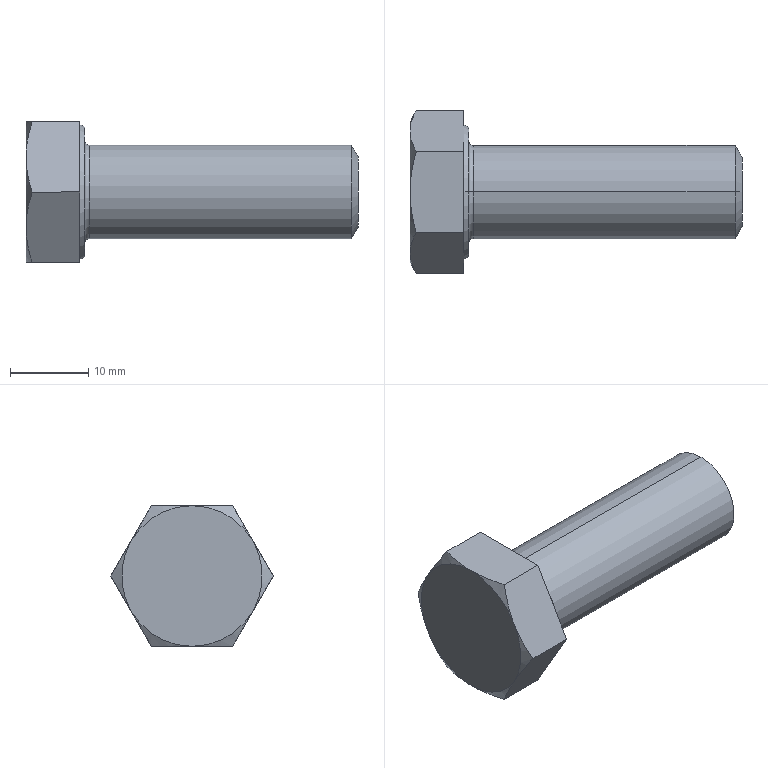Part | SolidWorks | features RevCut 3, Extrusion 1, Fillet 1, LPattern 1, Revolution 1 | 1 solid | 24 faces | box 42.5 x 20.785 x 18 mm | volume 6004 mm3 | cone 10 | plane 10 | torus 2 | cylinder 2 | commonest cylinder face diameters 12 x2
STEP:
#1=CARTESIAN_POINT('',(42.5,0.,4.484));
#2=VERTEX_POINT('',#1);
#3=CARTESIAN_POINT('',(42.5,0.,-4.484));
#4=VERTEX_POINT('',#3);
#5=CARTESIAN_POINT('',(42.5,0.,0.));
#6=DIRECTION('',(-1.,0.,0.));
#7=DIRECTION('',(0.,0.,1.));
#8=AXIS2_PLACEMENT_3D('',#5,#6,#7);
#9=CIRCLE('',#8,4.484);
#10=EDGE_CURVE('',#2,#4,#9,.T.);
#11=ORIENTED_EDGE('',*,*,#10,.T.);
#12=CARTESIAN_POINT('',(41.625,0.,-6.));
#13=VERTEX_POINT('',#12);
#14=CARTESIAN_POINT('',(41.625,0.,-6.));
#15=DIRECTION('',(-0.5,0.,-0.866));
#16=VECTOR('',#15,1000.);
#17=LINE('',#14,#16);
#18=EDGE_CURVE('',#4,#13,#17,.T.);
#19=ORIENTED_EDGE('',*,*,#18,.T.);
#20=CARTESIAN_POINT('',(41.625,0.,6.));
#21=VERTEX_POINT('',#20);
#22=CARTESIAN_POINT('',(41.625,0.,0.));
#23=DIRECTION('',(-1.,0.,0.));
#24=DIRECTION('',(0.,0.,1.));
#25=AXIS2_PLACEMENT_3D('',#22,#23,#24);
#26=CIRCLE('',#25,6.);
#27=EDGE_CURVE('',#21,#13,#26,.T.);
#28=ORIENTED_EDGE('',*,*,#27,.F.);
#29=CARTESIAN_POINT('',(41.625,0.,6.));
#30=DIRECTION('',(-0.5,0.,0.866));
#31=VECTOR('',#30,1000.);
#32=LINE('',#29,#31);
#33=EDGE_CURVE('',#2,#21,#32,.T.);
#34=ORIENTED_EDGE('',*,*,#33,.F.);
#35=EDGE_LOOP('',(#11,#19,#28,#34));
#36=FACE_OUTER_BOUND('',#35,.T.);
#37=CARTESIAN_POINT('',(41.625,0.,0.));
#38=DIRECTION('',(-1.,0.,0.));
#39=DIRECTION('',(0.,0.,1.));
#40=AXIS2_PLACEMENT_3D('',#37,#38,#39);
#41=CONICAL_SURFACE('',#40,6.,1.047);
#42=ADVANCED_FACE('',(#36),#41,.T.);
#43=CARTESIAN_POINT('',(8.1,0.,6.));
#44=VERTEX_POINT('',#43);
#45=CARTESIAN_POINT('',(8.1,0.,-6.));
#46=VERTEX_POINT('',#45);
#47=CARTESIAN_POINT('',(8.1,0.,0.));
#48=DIRECTION('',(1.,0.,0.));
#49=DIRECTION('',(0.,0.,-1.));
#50=AXIS2_PLACEMENT_3D('',#47,#48,#49);
#51=CIRCLE('',#50,6.);
#52=EDGE_CURVE('',#44,#46,#51,.T.);
#53=ORIENTED_EDGE('',*,*,#52,.F.);
#54=CARTESIAN_POINT('',(7.5,0.,6.6));
#55=VERTEX_POINT('',#54);
#56=CARTESIAN_POINT('',(8.1,0.,6.6));
#57=DIRECTION('',(0.,1.,0.));
#58=DIRECTION('',(0.,0.,1.));
#59=AXIS2_PLACEMENT_3D('',#56,#57,#58);
#60=CIRCLE('',#59,0.6);
#61=EDGE_CURVE('',#44,#55,#60,.T.);
#62=ORIENTED_EDGE('',*,*,#61,.T.);
#63=CARTESIAN_POINT('',(7.5,0.,-6.6));
#64=VERTEX_POINT('',#63);
#65=CARTESIAN_POINT('',(7.5,0.,0.));
#66=DIRECTION('',(-1.,0.,0.));
#67=DIRECTION('',(0.,0.,-1.));
#68=AXIS2_PLACEMENT_3D('',#65,#66,#67);
#69=CIRCLE('',#68,6.6);
#70=EDGE_CURVE('',#64,#55,#69,.T.);
#71=ORIENTED_EDGE('',*,*,#70,.F.);
#72=CARTESIAN_POINT('',(8.1,0.,-6.6));
#73=DIRECTION('',(0.,-1.,0.));
#74=DIRECTION('',(0.,0.,-1.));
#75=AXIS2_PLACEMENT_3D('',#72,#73,#74);
#76=CIRCLE('',#75,0.6);
#77=EDGE_CURVE('',#46,#64,#76,.T.);
#78=ORIENTED_EDGE('',*,*,#77,.F.);
#79=EDGE_LOOP('',(#53,#62,#71,#78));
#80=FACE_OUTER_BOUND('',#79,.T.);
#81=CARTESIAN_POINT('',(8.1,0.,0.));
#82=DIRECTION('',(1.,0.,0.));
#83=DIRECTION('',(0.,0.,-1.));
#84=AXIS2_PLACEMENT_3D('',#81,#82,#83);
#85=TOROIDAL_SURFACE('',#84,6.6,0.6);
#86=ADVANCED_FACE('',(#80),#85,.F.);
#87=CARTESIAN_POINT('',(7.5,0.,8.315));
#88=VERTEX_POINT('',#87);
#89=CARTESIAN_POINT('',(7.5,0.,-8.315));
#90=VERTEX_POINT('',#89);
#91=CARTESIAN_POINT('',(7.5,0.,0.));
#92=DIRECTION('',(-1.,0.,0.));
#93=DIRECTION('',(0.,0.,1.));
#94=AXIS2_PLACEMENT_3D('',#91,#92,#93);
#95=CIRCLE('',#94,8.315);
#96=EDGE_CURVE('',#88,#90,#95,.T.);
#97=ORIENTED_EDGE('',*,*,#96,.T.);
#98=CARTESIAN_POINT('',(6.9,0.,-8.661));
#99=VERTEX_POINT('',#98);
#100=CARTESIAN_POINT('',(6.9,0.,-8.661));
#101=DIRECTION('',(-0.866,0.,-0.5));
#102=VECTOR('',#101,1000.);
#103=LINE('',#100,#102);
#104=EDGE_CURVE('',#90,#99,#103,.T.);
#105=ORIENTED_EDGE('',*,*,#104,.T.);
#106=CARTESIAN_POINT('',(6.9,0.,8.661));
#107=VERTEX_POINT('',#106);
#108=CARTESIAN_POINT('',(6.9,0.,0.));
#109=DIRECTION('',(-1.,0.,0.));
#110=DIRECTION('',(0.,0.,1.));
#111=AXIS2_PLACEMENT_3D('',#108,#109,#110);
#112=CIRCLE('',#111,8.661);
#113=EDGE_CURVE('',#107,#99,#112,.T.);
#114=ORIENTED_EDGE('',*,*,#113,.F.);
#115=CARTESIAN_POINT('',(6.9,0.,8.661));
#116=DIRECTION('',(-0.866,0.,0.5));
#117=VECTOR('',#116,1000.);
#118=LINE('',#115,#117);
#119=EDGE_CURVE('',#88,#107,#118,.T.);
#120=ORIENTED_EDGE('',*,*,#119,.F.);
#121=EDGE_LOOP('',(#97,#105,#114,#120));
#122=FACE_OUTER_BOUND('',#121,.T.);
#123=CARTESIAN_POINT('',(6.9,0.,0.));
#124=DIRECTION('',(-1.,0.,0.));
#125=DIRECTION('',(0.,0.,1.));
#126=AXIS2_PLACEMENT_3D('',#123,#124,#125);
#127=CONICAL_SURFACE('',#126,8.661,0.5236);
#128=ADVANCED_FACE('',(#122),#127,.T.);
#129=ORIENTED_EDGE('',*,*,#27,.T.);
#130=CARTESIAN_POINT('',(0.,0.,-6.));
#131=DIRECTION('',(-1.,0.,0.));
#132=VECTOR('',#131,1000.);
#133=LINE('',#130,#132);
#134=EDGE_CURVE('',#13,#46,#133,.T.);
#135=ORIENTED_EDGE('',*,*,#134,.T.);
#136=CARTESIAN_POINT('',(8.1,0.,0.));
#137=DIRECTION('',(1.,0.,0.));
#138=DIRECTION('',(0.,0.,-1.));
#139=AXIS2_PLACEMENT_3D('',#136,#137,#138);
#140=CIRCLE('',#139,6.);
#141=EDGE_CURVE('',#46,#44,#140,.T.);
#142=ORIENTED_EDGE('',*,*,#141,.T.);
#143=CARTESIAN_POINT('',(0.,0.,6.));
#144=DIRECTION('',(-1.,0.,0.));
#145=VECTOR('',#144,1000.);
#146=LINE('',#143,#145);
#147=EDGE_CURVE('',#21,#44,#146,.T.);
#148=ORIENTED_EDGE('',*,*,#147,.F.);
#149=EDGE_LOOP('',(#129,#135,#142,#148));
#150=FACE_OUTER_BOUND('',#149,.T.);
#151=CARTESIAN_POINT('',(0.,0.,0.));
#152=DIRECTION('',(-1.,0.,0.));
#153=DIRECTION('',(0.,0.,1.));
#154=AXIS2_PLACEMENT_3D('',#151,#152,#153);
#155=CYLINDRICAL_SURFACE('',#154,6.);
#156=ADVANCED_FACE('',(#150),#155,.T.);
#157=ORIENTED_EDGE('',*,*,#134,.F.);
#158=CARTESIAN_POINT('',(41.625,0.,0.));
#159=DIRECTION('',(-1.,0.,0.));
#160=DIRECTION('',(0.,0.,1.));
#161=AXIS2_PLACEMENT_3D('',#158,#159,#160);
#162=CIRCLE('',#161,6.);
#163=EDGE_CURVE('',#13,#21,#162,.T.);
#164=ORIENTED_EDGE('',*,*,#163,.T.);
#165=ORIENTED_EDGE('',*,*,#147,.T.);
#166=ORIENTED_EDGE('',*,*,#52,.T.);
#167=EDGE_LOOP('',(#157,#164,#165,#166));
#168=FACE_OUTER_BOUND('',#167,.T.);
#169=CARTESIAN_POINT('',(0.,0.,0.));
#170=DIRECTION('',(-1.,0.,0.));
#171=DIRECTION('',(0.,0.,1.));
#172=AXIS2_PLACEMENT_3D('',#169,#170,#171);
#173=CYLINDRICAL_SURFACE('',#172,6.);
#174=ADVANCED_FACE('',(#168),#173,.T.);
#175=CARTESIAN_POINT('',(6.9,5.196,-9.));
#176=VERTEX_POINT('',#175);
#177=CARTESIAN_POINT('',(6.9,10.392,0.));
#178=VERTEX_POINT('',#177);
#179=CARTESIAN_POINT('',(6.9,5.196,-9.));
#180=DIRECTION('',(0.,0.5,0.866));
#181=VECTOR('',#180,1000.);
#182=LINE('',#179,#181);
#183=EDGE_CURVE('',#176,#178,#182,.T.);
#184=ORIENTED_EDGE('',*,*,#183,.F.);
#185=CARTESIAN_POINT('',(0.8038,5.196,-9.));
#186=VERTEX_POINT('',#185);
#187=CARTESIAN_POINT('',(7.5,5.196,-9.));
#188=DIRECTION('',(-1.,0.,0.));
#189=VECTOR('',#188,1000.);
#190=LINE('',#187,#189);
#191=EDGE_CURVE('',#176,#186,#190,.T.);
#192=ORIENTED_EDGE('',*,*,#191,.T.);
#193=CARTESIAN_POINT('',(0.,7.794,-4.5));
#194=VERTEX_POINT('',#193);
#195=CARTESIAN_POINT('',(0.,7.794,-4.5));
#196=CARTESIAN_POINT('',(0.,7.574,-4.882));
#197=CARTESIAN_POINT('',(0.019,7.352,-5.266));
#198=CARTESIAN_POINT('',(0.09253,6.914,-6.024));
#199=CARTESIAN_POINT('',(0.147,6.697,-6.401));
#200=CARTESIAN_POINT('',(0.357,6.048,-7.525));
#201=CARTESIAN_POINT('',(0.5591,5.62,-8.266));
#202=CARTESIAN_POINT('',(0.8038,5.196,-9.));
#203=B_SPLINE_CURVE_WITH_KNOTS('',3,(#195,#196,#197,#198,#199,#200,#201,#202),.UNSPECIFIED.,.F.,.F.,(4,2,2,4),(0.005258,0.006567,0.007877,0.0105),.UNSPECIFIED.);
#204=EDGE_CURVE('',#194,#186,#203,.T.);
#205=ORIENTED_EDGE('',*,*,#204,.F.);
#206=CARTESIAN_POINT('',(0.8038,10.392,0.));
#207=VERTEX_POINT('',#206);
#208=CARTESIAN_POINT('',(0.8038,10.392,0.));
#209=CARTESIAN_POINT('',(0.5585,9.967,-0.7361));
#210=CARTESIAN_POINT('',(0.3563,9.539,-1.478));
#211=CARTESIAN_POINT('',(0.07661,8.674,-2.976));
#212=CARTESIAN_POINT('',(0.,8.237,-3.733));
#213=CARTESIAN_POINT('',(0.,7.794,-4.5));
#214=B_SPLINE_CURVE_WITH_KNOTS('',3,(#208,#209,#210,#211,#212,#213),.UNSPECIFIED.,.F.,.F.,(4,2,4),(0.000000238,0.002629,0.005258),.UNSPECIFIED.);
#215=EDGE_CURVE('',#207,#194,#214,.T.);
#216=ORIENTED_EDGE('',*,*,#215,.F.);
#217=CARTESIAN_POINT('',(7.5,10.392,0.));
#218=DIRECTION('',(-1.,0.,0.));
#219=VECTOR('',#218,1000.);
#220=LINE('',#217,#219);
#221=EDGE_CURVE('',#178,#207,#220,.T.);
#222=ORIENTED_EDGE('',*,*,#221,.F.);
#223=EDGE_LOOP('',(#184,#192,#205,#216,#222));
#224=FACE_OUTER_BOUND('',#223,.T.);
#225=CARTESIAN_POINT('',(7.5,5.196,-9.));
#226=DIRECTION('',(0.,-0.866,0.5));
#227=DIRECTION('',(0.,-0.5,-0.866));
#228=AXIS2_PLACEMENT_3D('',#225,#226,#227);
#229=PLANE('',#228);
#230=ADVANCED_FACE('',(#224),#229,.F.);
#231=CARTESIAN_POINT('',(6.9,5.196,9.));
#232=VERTEX_POINT('',#231);
#233=CARTESIAN_POINT('',(6.9,10.392,0.));
#234=DIRECTION('',(0.,-0.5,0.866));
#235=VECTOR('',#234,1000.);
#236=LINE('',#233,#235);
#237=EDGE_CURVE('',#178,#232,#236,.T.);
#238=ORIENTED_EDGE('',*,*,#237,.F.);
#239=ORIENTED_EDGE('',*,*,#221,.T.);
#240=CARTESIAN_POINT('',(0.,7.794,4.5));
#241=VERTEX_POINT('',#240);
#242=CARTESIAN_POINT('',(0.,7.794,4.5));
#243=CARTESIAN_POINT('',(0.,8.015,4.118));
#244=CARTESIAN_POINT('',(0.019,8.236,3.734));
#245=CARTESIAN_POINT('',(0.09253,8.674,2.976));
#246=CARTESIAN_POINT('',(0.147,8.892,2.599));
#247=CARTESIAN_POINT('',(0.357,9.541,1.475));
#248=CARTESIAN_POINT('',(0.5591,9.968,0.7343));
#249=CARTESIAN_POINT('',(0.8038,10.392,0.));
#250=B_SPLINE_CURVE_WITH_KNOTS('',3,(#242,#243,#244,#245,#246,#247,#248,#249),.UNSPECIFIED.,.F.,.F.,(4,2,2,4),(0.005258,0.006567,0.007877,0.0105),.UNSPECIFIED.);
#251=EDGE_CURVE('',#241,#207,#250,.T.);
#252=ORIENTED_EDGE('',*,*,#251,.F.);
#253=CARTESIAN_POINT('',(0.8038,5.196,9.));
#254=VERTEX_POINT('',#253);
#255=CARTESIAN_POINT('',(0.8038,5.196,9.));
#256=CARTESIAN_POINT('',(0.5585,5.621,8.264));
#257=CARTESIAN_POINT('',(0.3563,6.049,7.522));
#258=CARTESIAN_POINT('',(0.07661,6.914,6.024));
#259=CARTESIAN_POINT('',(0.,7.352,5.267));
#260=CARTESIAN_POINT('',(0.,7.794,4.5));
#261=B_SPLINE_CURVE_WITH_KNOTS('',3,(#255,#256,#257,#258,#259,#260),.UNSPECIFIED.,.F.,.F.,(4,2,4),(0.000000238,0.002629,0.005258),.UNSPECIFIED.);
#262=EDGE_CURVE('',#254,#241,#261,.T.);
#263=ORIENTED_EDGE('',*,*,#262,.F.);
#264=CARTESIAN_POINT('',(7.5,5.196,9.));
#265=DIRECTION('',(-1.,0.,0.));
#266=VECTOR('',#265,1000.);
#267=LINE('',#264,#266);
#268=EDGE_CURVE('',#232,#254,#267,.T.);
#269=ORIENTED_EDGE('',*,*,#268,.F.);
#270=EDGE_LOOP('',(#238,#239,#252,#263,#269));
#271=FACE_OUTER_BOUND('',#270,.T.);
#272=CARTESIAN_POINT('',(7.5,10.392,0.));
#273=DIRECTION('',(0.,-0.866,-0.5));
#274=DIRECTION('',(0.,0.5,-0.866));
#275=AXIS2_PLACEMENT_3D('',#272,#273,#274);
#276=PLANE('',#275);
#277=ADVANCED_FACE('',(#271),#276,.F.);
#278=CARTESIAN_POINT('',(6.9,-5.196,9.));
#279=VERTEX_POINT('',#278);
#280=CARTESIAN_POINT('',(6.9,5.196,9.));
#281=DIRECTION('',(0.,-1.,0.));
#282=VECTOR('',#281,1000.);
#283=LINE('',#280,#282);
#284=EDGE_CURVE('',#232,#279,#283,.T.);
#285=ORIENTED_EDGE('',*,*,#284,.F.);
#286=ORIENTED_EDGE('',*,*,#268,.T.);
#287=CARTESIAN_POINT('',(0.,0.,9.));
#288=VERTEX_POINT('',#287);
#289=CARTESIAN_POINT('',(0.,0.,9.));
#290=CARTESIAN_POINT('',(0.,0.4401,9.));
#291=CARTESIAN_POINT('',(0.01885,0.8832,9.));
#292=CARTESIAN_POINT('',(0.09319,1.767,9.));
#293=CARTESIAN_POINT('',(0.1482,2.204,9.));
#294=CARTESIAN_POINT('',(0.3593,3.505,9.));
#295=CARTESIAN_POINT('',(0.5612,4.356,9.));
#296=CARTESIAN_POINT('',(0.8038,5.196,9.));
#297=B_SPLINE_CURVE_WITH_KNOTS('',3,(#289,#290,#291,#292,#293,#294,#295,#296),.UNSPECIFIED.,.F.,.F.,(4,2,2,4),(0.01498,0.0163,0.01761,0.02025),.UNSPECIFIED.);
#298=EDGE_CURVE('',#288,#254,#297,.T.);
#299=ORIENTED_EDGE('',*,*,#298,.F.);
#300=CARTESIAN_POINT('',(0.8038,-5.196,9.));
#301=VERTEX_POINT('',#300);
#302=CARTESIAN_POINT('',(0.8038,-5.196,9.));
#303=CARTESIAN_POINT('',(0.5595,-4.35,9.));
#304=CARTESIAN_POINT('',(0.3552,-3.485,9.));
#305=CARTESIAN_POINT('',(0.07569,-1.752,9.));
#306=CARTESIAN_POINT('',(0.,-0.8794,9.));
#307=CARTESIAN_POINT('',(0.,0.,9.));
#308=B_SPLINE_CURVE_WITH_KNOTS('',3,(#302,#303,#304,#305,#306,#307),.UNSPECIFIED.,.F.,.F.,(4,2,4),(0.00972,0.01235,0.01498),.UNSPECIFIED.);
#309=EDGE_CURVE('',#301,#288,#308,.T.);
#310=ORIENTED_EDGE('',*,*,#309,.F.);
#311=CARTESIAN_POINT('',(7.5,-5.196,9.));
#312=DIRECTION('',(-1.,0.,0.));
#313=VECTOR('',#312,1000.);
#314=LINE('',#311,#313);
#315=EDGE_CURVE('',#279,#301,#314,.T.);
#316=ORIENTED_EDGE('',*,*,#315,.F.);
#317=EDGE_LOOP('',(#285,#286,#299,#310,#316));
#318=FACE_OUTER_BOUND('',#317,.T.);
#319=CARTESIAN_POINT('',(7.5,5.196,9.));
#320=DIRECTION('',(0.,0.,-1.));
#321=DIRECTION('',(0.,1.,0.));
#322=AXIS2_PLACEMENT_3D('',#319,#320,#321);
#323=PLANE('',#322);
#324=ADVANCED_FACE('',(#318),#323,.F.);
#325=CARTESIAN_POINT('',(6.9,-10.392,0.));
#326=VERTEX_POINT('',#325);
#327=CARTESIAN_POINT('',(6.9,-10.392,0.));
#328=DIRECTION('',(0.,-0.5,-0.866));
#329=VECTOR('',#328,1000.);
#330=LINE('',#327,#329);
#331=EDGE_CURVE('',#279,#326,#330,.T.);
#332=ORIENTED_EDGE('',*,*,#331,.F.);
#333=ORIENTED_EDGE('',*,*,#315,.T.);
#334=CARTESIAN_POINT('',(0.,-7.794,4.5));
#335=VERTEX_POINT('',#334);
#336=CARTESIAN_POINT('',(0.,-7.794,4.5));
#337=CARTESIAN_POINT('',(0.,-7.574,4.882));
#338=CARTESIAN_POINT('',(0.019,-7.352,5.266));
#339=CARTESIAN_POINT('',(0.09253,-6.914,6.024));
#340=CARTESIAN_POINT('',(0.147,-6.697,6.401));
#341=CARTESIAN_POINT('',(0.357,-6.048,7.525));
#342=CARTESIAN_POINT('',(0.5591,-5.62,8.266));
#343=CARTESIAN_POINT('',(0.8038,-5.196,9.));
#344=B_SPLINE_CURVE_WITH_KNOTS('',3,(#336,#337,#338,#339,#340,#341,#342,#343),.UNSPECIFIED.,.F.,.F.,(4,2,2,4),(0.005258,0.006567,0.007877,0.0105),.UNSPECIFIED.);
#345=EDGE_CURVE('',#335,#301,#344,.T.);
#346=ORIENTED_EDGE('',*,*,#345,.F.);
#347=CARTESIAN_POINT('',(0.8038,-10.392,0.));
#348=VERTEX_POINT('',#347);
#349=CARTESIAN_POINT('',(0.8038,-10.392,0.));
#350=CARTESIAN_POINT('',(0.5585,-9.967,0.7361));
#351=CARTESIAN_POINT('',(0.3563,-9.539,1.478));
#352=CARTESIAN_POINT('',(0.07661,-8.674,2.976));
#353=CARTESIAN_POINT('',(0.,-8.237,3.733));
#354=CARTESIAN_POINT('',(0.,-7.794,4.5));
#355=B_SPLINE_CURVE_WITH_KNOTS('',3,(#349,#350,#351,#352,#353,#354),.UNSPECIFIED.,.F.,.F.,(4,2,4),(0.000000238,0.002629,0.005258),.UNSPECIFIED.);
#356=EDGE_CURVE('',#348,#335,#355,.T.);
#357=ORIENTED_EDGE('',*,*,#356,.F.);
#358=CARTESIAN_POINT('',(7.5,-10.392,0.));
#359=DIRECTION('',(-1.,0.,0.));
#360=VECTOR('',#359,1000.);
#361=LINE('',#358,#360);
#362=EDGE_CURVE('',#326,#348,#361,.T.);
#363=ORIENTED_EDGE('',*,*,#362,.F.);
#364=EDGE_LOOP('',(#332,#333,#346,#357,#363));
#365=FACE_OUTER_BOUND('',#364,.T.);
#366=CARTESIAN_POINT('',(7.5,-10.392,0.));
#367=DIRECTION('',(0.,0.866,-0.5));
#368=DIRECTION('',(0.,0.5,0.866));
#369=AXIS2_PLACEMENT_3D('',#366,#367,#368);
#370=PLANE('',#369);
#371=ADVANCED_FACE('',(#365),#370,.F.);
#372=CARTESIAN_POINT('',(6.9,-5.196,-9.));
#373=VERTEX_POINT('',#372);
#374=CARTESIAN_POINT('',(6.9,-5.196,-9.));
#375=DIRECTION('',(0.,0.5,-0.866));
#376=VECTOR('',#375,1000.);
#377=LINE('',#374,#376);
#378=EDGE_CURVE('',#326,#373,#377,.T.);
#379=ORIENTED_EDGE('',*,*,#378,.F.);
#380=ORIENTED_EDGE('',*,*,#362,.T.);
#381=CARTESIAN_POINT('',(0.,-7.794,-4.5));
#382=VERTEX_POINT('',#381);
#383=CARTESIAN_POINT('',(0.,-7.794,-4.5));
#384=CARTESIAN_POINT('',(0.,-8.015,-4.118));
#385=CARTESIAN_POINT('',(0.019,-8.236,-3.734));
#386=CARTESIAN_POINT('',(0.09253,-8.674,-2.976));
#387=CARTESIAN_POINT('',(0.147,-8.892,-2.599));
#388=CARTESIAN_POINT('',(0.357,-9.541,-1.475));
#389=CARTESIAN_POINT('',(0.5591,-9.968,-0.7343));
#390=CARTESIAN_POINT('',(0.8038,-10.392,0.));
#391=B_SPLINE_CURVE_WITH_KNOTS('',3,(#383,#384,#385,#386,#387,#388,#389,#390),.UNSPECIFIED.,.F.,.F.,(4,2,2,4),(0.005258,0.006567,0.007877,0.0105),.UNSPECIFIED.);
#392=EDGE_CURVE('',#382,#348,#391,.T.);
#393=ORIENTED_EDGE('',*,*,#392,.F.);
#394=CARTESIAN_POINT('',(0.8038,-5.196,-9.));
#395=VERTEX_POINT('',#394);
#396=CARTESIAN_POINT('',(0.8038,-5.196,-9.));
#397=CARTESIAN_POINT('',(0.5585,-5.621,-8.264));
#398=CARTESIAN_POINT('',(0.3563,-6.049,-7.522));
#399=CARTESIAN_POINT('',(0.07661,-6.914,-6.024));
#400=CARTESIAN_POINT('',(0.,-7.352,-5.267));
#401=CARTESIAN_POINT('',(0.,-7.794,-4.5));
#402=B_SPLINE_CURVE_WITH_KNOTS('',3,(#396,#397,#398,#399,#400,#401),.UNSPECIFIED.,.F.,.F.,(4,2,4),(0.000000238,0.002629,0.005258),.UNSPECIFIED.);
#403=EDGE_CURVE('',#395,#382,#402,.T.);
#404=ORIENTED_EDGE('',*,*,#403,.F.);
#405=CARTESIAN_POINT('',(7.5,-5.196,-9.));
#406=DIRECTION('',(-1.,0.,0.));
#407=VECTOR('',#406,1000.);
#408=LINE('',#405,#407);
#409=EDGE_CURVE('',#373,#395,#408,.T.);
#410=ORIENTED_EDGE('',*,*,#409,.F.);
#411=EDGE_LOOP('',(#379,#380,#393,#404,#410));
#412=FACE_OUTER_BOUND('',#411,.T.);
#413=CARTESIAN_POINT('',(7.5,-5.196,-9.));
#414=DIRECTION('',(0.,0.866,0.5));
#415=DIRECTION('',(0.,-0.5,0.866));
#416=AXIS2_PLACEMENT_3D('',#413,#414,#415);
#417=PLANE('',#416);
#418=ADVANCED_FACE('',(#412),#417,.F.);
#419=CARTESIAN_POINT('',(6.9,5.196,-9.));
#420=DIRECTION('',(0.,1.,0.));
#421=VECTOR('',#420,1000.);
#422=LINE('',#419,#421);
#423=EDGE_CURVE('',#373,#176,#422,.T.);
#424=ORIENTED_EDGE('',*,*,#423,.F.);
#425=ORIENTED_EDGE('',*,*,#409,.T.);
#426=CARTESIAN_POINT('',(0.,0.,-9.));
#427=VERTEX_POINT('',#426);
#428=CARTESIAN_POINT('',(0.,0.,-9.));
#429=CARTESIAN_POINT('',(0.,-0.8794,-9.));
#430=CARTESIAN_POINT('',(0.07569,-1.752,-9.));
#431=CARTESIAN_POINT('',(0.3552,-3.485,-9.));
#432=CARTESIAN_POINT('',(0.5595,-4.35,-9.));
#433=CARTESIAN_POINT('',(0.8038,-5.196,-9.));
#434=B_SPLINE_CURVE_WITH_KNOTS('',3,(#428,#429,#430,#431,#432,#433),.UNSPECIFIED.,.F.,.F.,(4,2,4),(0.03045,0.03308,0.03571),.UNSPECIFIED.);
#435=EDGE_CURVE('',#427,#395,#434,.T.);
#436=ORIENTED_EDGE('',*,*,#435,.F.);
#437=CARTESIAN_POINT('',(0.8038,5.196,-9.));
#438=CARTESIAN_POINT('',(0.5612,4.356,-9.));
#439=CARTESIAN_POINT('',(0.3593,3.505,-9.));
#440=CARTESIAN_POINT('',(0.1482,2.204,-9.));
#441=CARTESIAN_POINT('',(0.09319,1.767,-9.));
#442=CARTESIAN_POINT('',(0.01885,0.8832,-9.));
#443=CARTESIAN_POINT('',(0.,0.4401,-9.));
#444=CARTESIAN_POINT('',(0.,0.,-9.));
#445=B_SPLINE_CURVE_WITH_KNOTS('',3,(#437,#438,#439,#440,#441,#442,#443,#444),.UNSPECIFIED.,.F.,.F.,(4,2,2,4),(0.02519,0.02782,0.02914,0.03045),.UNSPECIFIED.);
#446=EDGE_CURVE('',#186,#427,#445,.T.);
#447=ORIENTED_EDGE('',*,*,#446,.F.);
#448=ORIENTED_EDGE('',*,*,#191,.F.);
#449=EDGE_LOOP('',(#424,#425,#436,#447,#448));
#450=FACE_OUTER_BOUND('',#449,.T.);
#451=CARTESIAN_POINT('',(7.5,5.196,-9.));
#452=DIRECTION('',(0.,0.,1.));
#453=DIRECTION('',(0.,-1.,0.));
#454=AXIS2_PLACEMENT_3D('',#451,#452,#453);
#455=PLANE('',#454);
#456=ADVANCED_FACE('',(#450),#455,.F.);
#457=ORIENTED_EDGE('',*,*,#403,.T.);
#458=CARTESIAN_POINT('',(0.,0.,0.));
#459=DIRECTION('',(1.,0.,0.));
#460=DIRECTION('',(0.,0.,-1.));
#461=AXIS2_PLACEMENT_3D('',#458,#459,#460);
#462=CIRCLE('',#461,9.);
#463=EDGE_CURVE('',#382,#427,#462,.T.);
#464=ORIENTED_EDGE('',*,*,#463,.T.);
#465=ORIENTED_EDGE('',*,*,#435,.T.);
#466=EDGE_LOOP('',(#457,#464,#465));
#467=FACE_OUTER_BOUND('',#466,.T.);
#468=CARTESIAN_POINT('',(0.,0.,0.));
#469=DIRECTION('',(1.,0.,0.));
#470=DIRECTION('',(0.,0.,-1.));
#471=AXIS2_PLACEMENT_3D('',#468,#469,#470);
#472=CONICAL_SURFACE('',#471,9.,1.047);
#473=ADVANCED_FACE('',(#467),#472,.T.);
#474=ORIENTED_EDGE('',*,*,#356,.T.);
#475=CARTESIAN_POINT('',(0.,0.,0.));
#476=DIRECTION('',(1.,0.,0.));
#477=DIRECTION('',(0.,0.,-1.));
#478=AXIS2_PLACEMENT_3D('',#475,#476,#477);
#479=CIRCLE('',#478,9.);
#480=EDGE_CURVE('',#335,#382,#479,.T.);
#481=ORIENTED_EDGE('',*,*,#480,.T.);
#482=ORIENTED_EDGE('',*,*,#392,.T.);
#483=EDGE_LOOP('',(#474,#481,#482));
#484=FACE_OUTER_BOUND('',#483,.T.);
#485=CARTESIAN_POINT('',(0.,0.,0.));
#486=DIRECTION('',(1.,0.,0.));
#487=DIRECTION('',(0.,0.,-1.));
#488=AXIS2_PLACEMENT_3D('',#485,#486,#487);
#489=CONICAL_SURFACE('',#488,9.,1.047);
#490=ADVANCED_FACE('',(#484),#489,.T.);
#491=ORIENTED_EDGE('',*,*,#309,.T.);
#492=CARTESIAN_POINT('',(0.,0.,0.));
#493=DIRECTION('',(1.,0.,0.));
#494=DIRECTION('',(0.,0.,-1.));
#495=AXIS2_PLACEMENT_3D('',#492,#493,#494);
#496=CIRCLE('',#495,9.);
#497=EDGE_CURVE('',#288,#335,#496,.T.);
#498=ORIENTED_EDGE('',*,*,#497,.T.);
#499=ORIENTED_EDGE('',*,*,#345,.T.);
#500=EDGE_LOOP('',(#491,#498,#499));
#501=FACE_OUTER_BOUND('',#500,.T.);
#502=CARTESIAN_POINT('',(0.,0.,0.));
#503=DIRECTION('',(1.,0.,0.));
#504=DIRECTION('',(0.,0.,-1.));
#505=AXIS2_PLACEMENT_3D('',#502,#503,#504);
#506=CONICAL_SURFACE('',#505,9.,1.047);
#507=ADVANCED_FACE('',(#501),#506,.T.);
#508=ORIENTED_EDGE('',*,*,#298,.T.);
#509=ORIENTED_EDGE('',*,*,#262,.T.);
#510=CARTESIAN_POINT('',(0.,0.,0.));
#511=DIRECTION('',(-1.,0.,0.));
#512=DIRECTION('',(0.,0.,1.));
#513=AXIS2_PLACEMENT_3D('',#510,#511,#512);
#514=CIRCLE('',#513,9.);
#515=EDGE_CURVE('',#288,#241,#514,.T.);
#516=ORIENTED_EDGE('',*,*,#515,.F.);
#517=EDGE_LOOP('',(#508,#509,#516));
#518=FACE_OUTER_BOUND('',#517,.T.);
#519=CARTESIAN_POINT('',(0.,0.,0.));
#520=DIRECTION('',(1.,0.,0.));
#521=DIRECTION('',(0.,0.,-1.));
#522=AXIS2_PLACEMENT_3D('',#519,#520,#521);
#523=CONICAL_SURFACE('',#522,9.,1.047);
#524=ADVANCED_FACE('',(#518),#523,.T.);
#525=ORIENTED_EDGE('',*,*,#251,.T.);
#526=ORIENTED_EDGE('',*,*,#215,.T.);
#527=CARTESIAN_POINT('',(0.,0.,0.));
#528=DIRECTION('',(1.,0.,0.));
#529=DIRECTION('',(0.,0.,-1.));
#530=AXIS2_PLACEMENT_3D('',#527,#528,#529);
#531=CIRCLE('',#530,9.);
#532=EDGE_CURVE('',#194,#241,#531,.T.);
#533=ORIENTED_EDGE('',*,*,#532,.T.);
#534=EDGE_LOOP('',(#525,#526,#533));
#535=FACE_OUTER_BOUND('',#534,.T.);
#536=CARTESIAN_POINT('',(0.,0.,0.));
#537=DIRECTION('',(1.,0.,0.));
#538=DIRECTION('',(0.,0.,-1.));
#539=AXIS2_PLACEMENT_3D('',#536,#537,#538);
#540=CONICAL_SURFACE('',#539,9.,1.047);
#541=ADVANCED_FACE('',(#535),#540,.T.);
#542=ORIENTED_EDGE('',*,*,#204,.T.);
#543=ORIENTED_EDGE('',*,*,#446,.T.);
#544=CARTESIAN_POINT('',(0.,0.,0.));
#545=DIRECTION('',(1.,0.,0.));
#546=DIRECTION('',(0.,0.,-1.));
#547=AXIS2_PLACEMENT_3D('',#544,#545,#546);
#548=CIRCLE('',#547,9.);
#549=EDGE_CURVE('',#427,#194,#548,.T.);
#550=ORIENTED_EDGE('',*,*,#549,.T.);
#551=EDGE_LOOP('',(#542,#543,#550));
#552=FACE_OUTER_BOUND('',#551,.T.);
#553=CARTESIAN_POINT('',(0.,0.,0.));
#554=DIRECTION('',(1.,0.,0.));
#555=DIRECTION('',(0.,0.,-1.));
#556=AXIS2_PLACEMENT_3D('',#553,#554,#555);
#557=CONICAL_SURFACE('',#556,9.,1.047);
#558=ADVANCED_FACE('',(#552),#557,.T.);
#559=ORIENTED_EDGE('',*,*,#549,.F.);
#560=ORIENTED_EDGE('',*,*,#463,.F.);
#561=ORIENTED_EDGE('',*,*,#480,.F.);
#562=ORIENTED_EDGE('',*,*,#497,.F.);
#563=ORIENTED_EDGE('',*,*,#515,.T.);
#564=ORIENTED_EDGE('',*,*,#532,.F.);
#565=EDGE_LOOP('',(#559,#560,#561,#562,#563,#564));
#566=FACE_OUTER_BOUND('',#565,.T.);
#567=CARTESIAN_POINT('',(0.,10.392,0.));
#568=DIRECTION('',(1.,0.,0.));
#569=DIRECTION('',(0.,0.,-1.));
#570=AXIS2_PLACEMENT_3D('',#567,#568,#569);
#571=PLANE('',#570);
#572=ADVANCED_FACE('',(#566),#571,.F.);
#573=ORIENTED_EDGE('',*,*,#113,.T.);
#574=CARTESIAN_POINT('',(6.9,0.,0.));
#575=DIRECTION('',(-1.,0.,0.));
#576=DIRECTION('',(0.,0.,1.));
#577=AXIS2_PLACEMENT_3D('',#574,#575,#576);
#578=CIRCLE('',#577,8.661);
#579=EDGE_CURVE('',#99,#107,#578,.T.);
#580=ORIENTED_EDGE('',*,*,#579,.T.);
#581=EDGE_LOOP('',(#573,#580));
#582=FACE_BOUND('',#581,.T.);
#583=ORIENTED_EDGE('',*,*,#183,.T.);
#584=ORIENTED_EDGE('',*,*,#237,.T.);
#585=ORIENTED_EDGE('',*,*,#284,.T.);
#586=ORIENTED_EDGE('',*,*,#331,.T.);
#587=ORIENTED_EDGE('',*,*,#378,.T.);
#588=ORIENTED_EDGE('',*,*,#423,.T.);
#589=EDGE_LOOP('',(#583,#584,#585,#586,#587,#588));
#590=FACE_OUTER_BOUND('',#589,.T.);
#591=CARTESIAN_POINT('',(6.9,8.661,0.));
#592=DIRECTION('',(1.,0.,0.));
#593=DIRECTION('',(0.,0.,-1.));
#594=AXIS2_PLACEMENT_3D('',#591,#592,#593);
#595=PLANE('',#594);
#596=ADVANCED_FACE('',(#582,#590),#595,.T.);
#597=ORIENTED_EDGE('',*,*,#104,.F.);
#598=CARTESIAN_POINT('',(7.5,0.,0.));
#599=DIRECTION('',(-1.,0.,0.));
#600=DIRECTION('',(0.,0.,1.));
#601=AXIS2_PLACEMENT_3D('',#598,#599,#600);
#602=CIRCLE('',#601,8.315);
#603=EDGE_CURVE('',#90,#88,#602,.T.);
#604=ORIENTED_EDGE('',*,*,#603,.T.);
#605=ORIENTED_EDGE('',*,*,#119,.T.);
#606=ORIENTED_EDGE('',*,*,#579,.F.);
#607=EDGE_LOOP('',(#597,#604,#605,#606));
#608=FACE_OUTER_BOUND('',#607,.T.);
#609=CARTESIAN_POINT('',(6.9,0.,0.));
#610=DIRECTION('',(-1.,0.,0.));
#611=DIRECTION('',(0.,0.,1.));
#612=AXIS2_PLACEMENT_3D('',#609,#610,#611);
#613=CONICAL_SURFACE('',#612,8.661,0.5236);
#614=ADVANCED_FACE('',(#608),#613,.T.);
#615=ORIENTED_EDGE('',*,*,#70,.T.);
#616=CARTESIAN_POINT('',(7.5,0.,0.));
#617=DIRECTION('',(-1.,0.,0.));
#618=DIRECTION('',(0.,0.,-1.));
#619=AXIS2_PLACEMENT_3D('',#616,#617,#618);
#620=CIRCLE('',#619,6.6);
#621=EDGE_CURVE('',#55,#64,#620,.T.);
#622=ORIENTED_EDGE('',*,*,#621,.T.);
#623=EDGE_LOOP('',(#615,#622));
#624=FACE_BOUND('',#623,.T.);
#625=ORIENTED_EDGE('',*,*,#96,.F.);
#626=ORIENTED_EDGE('',*,*,#603,.F.);
#627=EDGE_LOOP('',(#625,#626));
#628=FACE_OUTER_BOUND('',#627,.T.);
#629=CARTESIAN_POINT('',(7.5,10.392,0.));
#630=DIRECTION('',(1.,0.,0.));
#631=DIRECTION('',(0.,0.,-1.));
#632=AXIS2_PLACEMENT_3D('',#629,#630,#631);
#633=PLANE('',#632);
#634=ADVANCED_FACE('',(#624,#628),#633,.T.);
#635=ORIENTED_EDGE('',*,*,#61,.F.);
#636=ORIENTED_EDGE('',*,*,#141,.F.);
#637=ORIENTED_EDGE('',*,*,#77,.T.);
#638=ORIENTED_EDGE('',*,*,#621,.F.);
#639=EDGE_LOOP('',(#635,#636,#637,#638));
#640=FACE_OUTER_BOUND('',#639,.T.);
#641=CARTESIAN_POINT('',(8.1,0.,0.));
#642=DIRECTION('',(1.,0.,0.));
#643=DIRECTION('',(0.,0.,-1.));
#644=AXIS2_PLACEMENT_3D('',#641,#642,#643);
#645=TOROIDAL_SURFACE('',#644,6.6,0.6);
#646=ADVANCED_FACE('',(#640),#645,.F.);
#647=ORIENTED_EDGE('',*,*,#18,.F.);
#648=CARTESIAN_POINT('',(42.5,0.,0.));
#649=DIRECTION('',(-1.,0.,0.));
#650=DIRECTION('',(0.,0.,1.));
#651=AXIS2_PLACEMENT_3D('',#648,#649,#650);
#652=CIRCLE('',#651,4.484);
#653=EDGE_CURVE('',#4,#2,#652,.T.);
#654=ORIENTED_EDGE('',*,*,#653,.T.);
#655=ORIENTED_EDGE('',*,*,#33,.T.);
#656=ORIENTED_EDGE('',*,*,#163,.F.);
#657=EDGE_LOOP('',(#647,#654,#655,#656));
#658=FACE_OUTER_BOUND('',#657,.T.);
#659=CARTESIAN_POINT('',(41.625,0.,0.));
#660=DIRECTION('',(-1.,0.,0.));
#661=DIRECTION('',(0.,0.,1.));
#662=AXIS2_PLACEMENT_3D('',#659,#660,#661);
#663=CONICAL_SURFACE('',#662,6.,1.047);
#664=ADVANCED_FACE('',(#658),#663,.T.);
#665=ORIENTED_EDGE('',*,*,#10,.F.);
#666=ORIENTED_EDGE('',*,*,#653,.F.);
#667=EDGE_LOOP('',(#665,#666));
#668=FACE_OUTER_BOUND('',#667,.T.);
#669=CARTESIAN_POINT('',(42.5,0.,0.));
#670=DIRECTION('',(-1.,0.,0.));
#671=DIRECTION('',(0.,0.,1.));
#672=AXIS2_PLACEMENT_3D('',#669,#670,#671);
#673=PLANE('',#672);
#674=ADVANCED_FACE('',(#668),#673,.F.);
#675=CLOSED_SHELL('',(#42,#86,#128,#156,#174,#230,#277,#324,#371,#418,#456,#473,#490,#507,#524,#541,#558,#572,#596,#614,#634,#646,#664,#674));
#676=MANIFOLD_SOLID_BREP('',#675);
#677=CARTESIAN_POINT('',(0.,0.,0.));
#678=DIRECTION('',(0.,0.,1.));
#679=DIRECTION('',(1.,0.,0.));
#680=AXIS2_PLACEMENT_3D('',#677,#678,#679);
#681=(LENGTH_UNIT()NAMED_UNIT(*)SI_UNIT(.MILLI.,.METRE.));
#682=UNCERTAINTY_MEASURE_WITH_UNIT(LENGTH_MEASURE(0.00001),#681,'','');
#683=(NAMED_UNIT(*)PLANE_ANGLE_UNIT()SI_UNIT($,.RADIAN.));
#684=(NAMED_UNIT(*)SI_UNIT($,.STERADIAN.)SOLID_ANGLE_UNIT());
#685=(GEOMETRIC_REPRESENTATION_CONTEXT(3)GLOBAL_UNCERTAINTY_ASSIGNED_CONTEXT((#682))GLOBAL_UNIT_ASSIGNED_CONTEXT((#681,#683,#684))REPRESENTATION_CONTEXT('',''));
#686=ADVANCED_BREP_SHAPE_REPRESENTATION('',(#676,#680),#685);